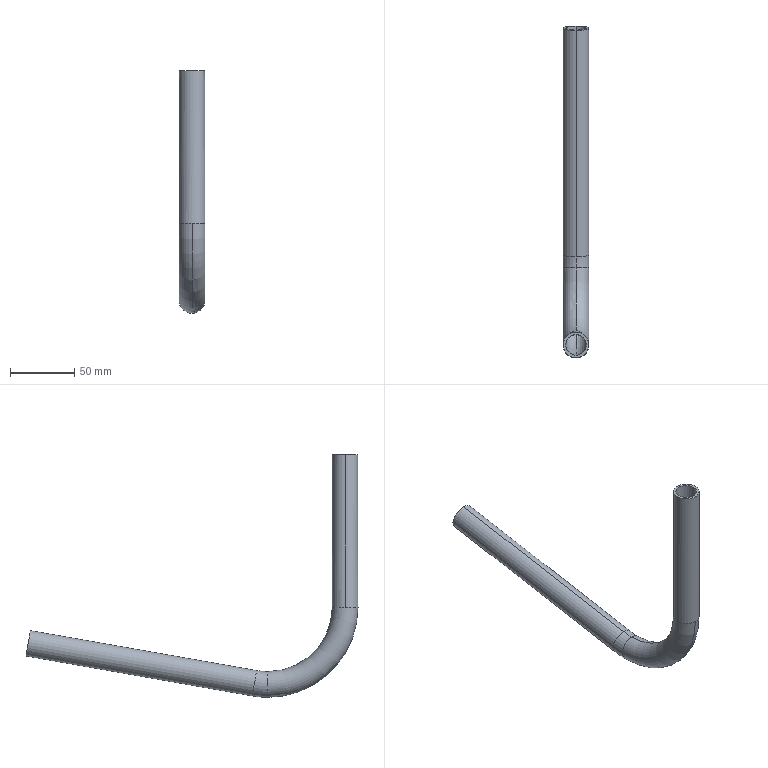Part | STEP file | Handlebar | 1 solid | 18 faces | box 20 x 257.938 x 188.495 mm | volume 45432 mm3 | torus 8 | cylinder 8 | plane 2 | commonest cylinder face diameters 16 x4 20 x4
STEP:
#1=CARTESIAN_POINT('',(0.,0.,0.));
#2=DIRECTION('',(0.,0.,1.));
#3=DIRECTION('',(1.,0.,0.));
#4=AXIS2_PLACEMENT_3D('',#1,#2,#3);
#5=CARTESIAN_POINT('',(0.,8.,-118.495));
#6=VERTEX_POINT('',#5);
#7=CARTESIAN_POINT('',(-8.,0.,-118.495));
#8=VERTEX_POINT('',#7);
#9=CARTESIAN_POINT('',(0.,0.,-118.495));
#10=DIRECTION('',(0.,0.,1.));
#11=DIRECTION('',(1.,0.,0.));
#12=AXIS2_PLACEMENT_3D('',#9,#10,#11);
#13=CIRCLE('',#12,8.);
#14=CARTESIAN_POINT('',(0.,60.,-118.495));
#15=DIRECTION('',(1.,0.,0.));
#16=DIRECTION('',(0.,0.,-1.));
#17=AXIS2_PLACEMENT_3D('',#14,#15,#16);
#18=TOROIDAL_SURFACE('',#17,60.,8.);
#19=CARTESIAN_POINT('',(4.712,1.571));
#20=DIRECTION('',(0.,1.));
#21=VECTOR('',#20,1.);
#22=LINE('',#19,#21);
#23=(GEOMETRIC_REPRESENTATION_CONTEXT(2)PARAMETRIC_REPRESENTATION_CONTEXT()REPRESENTATION_CONTEXT('',''));
#24=DEFINITIONAL_REPRESENTATION('',(#22),#23);
#25=PCURVE('',#18,#24);
#26=CARTESIAN_POINT('',(0.,0.,-118.495));
#27=DIRECTION('',(0.,0.,1.));
#28=DIRECTION('',(1.,0.,0.));
#29=AXIS2_PLACEMENT_3D('',#26,#27,#28);
#30=CYLINDRICAL_SURFACE('',#29,8.);
#31=CARTESIAN_POINT('',(0.,0.));
#32=DIRECTION('',(1.,0.));
#33=VECTOR('',#32,1.);
#34=LINE('',#31,#33);
#35=(GEOMETRIC_REPRESENTATION_CONTEXT(2)PARAMETRIC_REPRESENTATION_CONTEXT()REPRESENTATION_CONTEXT('',''));
#36=DEFINITIONAL_REPRESENTATION('',(#34),#35);
#37=PCURVE('',#30,#36);
#38=SURFACE_CURVE('',#13,(#25,#37),.PCURVE_S1.);
#39=EDGE_CURVE('',#6,#8,#38,.T.);
#40=ORIENTED_EDGE('',*,*,#39,.F.);
#41=CARTESIAN_POINT('',(0.,60.,-170.495));
#42=VERTEX_POINT('',#41);
#43=CARTESIAN_POINT('',(0.,60.,-118.495));
#44=DIRECTION('',(1.,0.,0.));
#45=DIRECTION('',(0.,0.,-1.));
#46=AXIS2_PLACEMENT_3D('',#43,#44,#45);
#47=CIRCLE('',#46,52.);
#48=CARTESIAN_POINT('',(0.,3.142));
#49=DIRECTION('',(1.,0.));
#50=VECTOR('',#49,1.);
#51=LINE('',#48,#50);
#52=(GEOMETRIC_REPRESENTATION_CONTEXT(2)PARAMETRIC_REPRESENTATION_CONTEXT()REPRESENTATION_CONTEXT('',''));
#53=DEFINITIONAL_REPRESENTATION('',(#51),#52);
#54=PCURVE('',#18,#53);
#55=CARTESIAN_POINT('',(0.,60.,-118.495));
#56=DIRECTION('',(1.,0.,0.));
#57=DIRECTION('',(0.,0.,-1.));
#58=AXIS2_PLACEMENT_3D('',#55,#56,#57);
#59=TOROIDAL_SURFACE('',#58,60.,8.);
#60=CARTESIAN_POINT('',(0.,3.142));
#61=DIRECTION('',(1.,0.));
#62=VECTOR('',#61,1.);
#63=LINE('',#60,#62);
#64=(GEOMETRIC_REPRESENTATION_CONTEXT(2)PARAMETRIC_REPRESENTATION_CONTEXT()REPRESENTATION_CONTEXT('',''));
#65=DEFINITIONAL_REPRESENTATION('',(#63),#64);
#66=PCURVE('',#59,#65);
#67=SURFACE_CURVE('',#47,(#54,#66),.PCURVE_S1.);
#68=EDGE_CURVE('',#6,#42,#67,.T.);
#69=ORIENTED_EDGE('',*,*,#68,.T.);
#70=CARTESIAN_POINT('',(0.,60.,-186.495));
#71=VERTEX_POINT('',#70);
#72=CARTESIAN_POINT('',(0.,60.,-178.495));
#73=DIRECTION('',(0.,-1.,0.));
#74=DIRECTION('',(0.,0.,-1.));
#75=AXIS2_PLACEMENT_3D('',#72,#73,#74);
#76=CIRCLE('',#75,8.);
#77=CARTESIAN_POINT('',(6.283,0.));
#78=DIRECTION('',(0.,1.));
#79=VECTOR('',#78,1.);
#80=LINE('',#77,#79);
#81=(GEOMETRIC_REPRESENTATION_CONTEXT(2)PARAMETRIC_REPRESENTATION_CONTEXT()REPRESENTATION_CONTEXT('',''));
#82=DEFINITIONAL_REPRESENTATION('',(#80),#81);
#83=PCURVE('',#18,#82);
#84=CARTESIAN_POINT('',(0.,60.,-118.495));
#85=DIRECTION('',(1.,0.,0.));
#86=DIRECTION('',(0.,0.,-1.));
#87=AXIS2_PLACEMENT_3D('',#84,#85,#86);
#88=TOROIDAL_SURFACE('',#87,60.,8.);
#89=CARTESIAN_POINT('',(0.,0.));
#90=DIRECTION('',(0.,1.));
#91=VECTOR('',#90,1.);
#92=LINE('',#89,#91);
#93=(GEOMETRIC_REPRESENTATION_CONTEXT(2)PARAMETRIC_REPRESENTATION_CONTEXT()REPRESENTATION_CONTEXT('',''));
#94=DEFINITIONAL_REPRESENTATION('',(#92),#93);
#95=PCURVE('',#88,#94);
#96=SURFACE_CURVE('',#76,(#83,#95),.PCURVE_S1.);
#97=EDGE_CURVE('',#42,#71,#96,.T.);
#98=ORIENTED_EDGE('',*,*,#97,.T.);
#99=CARTESIAN_POINT('',(0.,-8.,-118.495));
#100=VERTEX_POINT('',#99);
#101=CARTESIAN_POINT('',(0.,60.,-118.495));
#102=DIRECTION('',(1.,0.,0.));
#103=DIRECTION('',(0.,0.,-1.));
#104=AXIS2_PLACEMENT_3D('',#101,#102,#103);
#105=CIRCLE('',#104,68.);
#106=CARTESIAN_POINT('',(0.,6.283));
#107=DIRECTION('',(1.,0.));
#108=VECTOR('',#107,1.);
#109=LINE('',#106,#108);
#110=(GEOMETRIC_REPRESENTATION_CONTEXT(2)PARAMETRIC_REPRESENTATION_CONTEXT()REPRESENTATION_CONTEXT('',''));
#111=DEFINITIONAL_REPRESENTATION('',(#109),#110);
#112=PCURVE('',#18,#111);
#113=CARTESIAN_POINT('',(0.,0.));
#114=DIRECTION('',(1.,0.));
#115=VECTOR('',#114,1.);
#116=LINE('',#113,#115);
#117=(GEOMETRIC_REPRESENTATION_CONTEXT(2)PARAMETRIC_REPRESENTATION_CONTEXT()REPRESENTATION_CONTEXT('',''));
#118=DEFINITIONAL_REPRESENTATION('',(#116),#117);
#119=PCURVE('',#59,#118);
#120=SURFACE_CURVE('',#105,(#112,#119),.PCURVE_S1.);
#121=EDGE_CURVE('',#100,#71,#120,.T.);
#122=ORIENTED_EDGE('',*,*,#121,.F.);
#123=CARTESIAN_POINT('',(0.,0.,-118.495));
#124=DIRECTION('',(0.,0.,1.));
#125=DIRECTION('',(1.,0.,0.));
#126=AXIS2_PLACEMENT_3D('',#123,#124,#125);
#127=CIRCLE('',#126,8.);
#128=CARTESIAN_POINT('',(4.712,1.571));
#129=DIRECTION('',(0.,1.));
#130=VECTOR('',#129,1.);
#131=LINE('',#128,#130);
#132=(GEOMETRIC_REPRESENTATION_CONTEXT(2)PARAMETRIC_REPRESENTATION_CONTEXT()REPRESENTATION_CONTEXT('',''));
#133=DEFINITIONAL_REPRESENTATION('',(#131),#132);
#134=PCURVE('',#18,#133);
#135=CARTESIAN_POINT('',(0.,0.,-118.495));
#136=DIRECTION('',(0.,0.,1.));
#137=DIRECTION('',(1.,0.,0.));
#138=AXIS2_PLACEMENT_3D('',#135,#136,#137);
#139=CYLINDRICAL_SURFACE('',#138,8.);
#140=CARTESIAN_POINT('',(0.,0.));
#141=DIRECTION('',(1.,0.));
#142=VECTOR('',#141,1.);
#143=LINE('',#140,#142);
#144=(GEOMETRIC_REPRESENTATION_CONTEXT(2)PARAMETRIC_REPRESENTATION_CONTEXT()REPRESENTATION_CONTEXT('',''));
#145=DEFINITIONAL_REPRESENTATION('',(#143),#144);
#146=PCURVE('',#139,#145);
#147=SURFACE_CURVE('',#127,(#134,#146),.PCURVE_S1.);
#148=EDGE_CURVE('',#8,#100,#147,.T.);
#149=ORIENTED_EDGE('',*,*,#148,.F.);
#150=EDGE_LOOP('',(#40,#69,#98,#122,#149));
#151=FACE_BOUND('',#150,.F.);
#152=ADVANCED_FACE('',(#151),#18,.F.);
#153=CARTESIAN_POINT('',(0.,60.,-188.495));
#154=VERTEX_POINT('',#153);
#155=CARTESIAN_POINT('',(0.,60.,-168.495));
#156=VERTEX_POINT('',#155);
#157=CARTESIAN_POINT('',(0.,60.,-178.495));
#158=DIRECTION('',(0.,-1.,0.));
#159=DIRECTION('',(0.,0.,-1.));
#160=AXIS2_PLACEMENT_3D('',#157,#158,#159);
#161=CIRCLE('',#160,10.);
#162=CARTESIAN_POINT('',(0.,60.,-118.495));
#163=DIRECTION('',(1.,0.,0.));
#164=DIRECTION('',(0.,0.,-1.));
#165=AXIS2_PLACEMENT_3D('',#162,#163,#164);
#166=TOROIDAL_SURFACE('',#165,60.,10.);
#167=CARTESIAN_POINT('',(0.,0.));
#168=DIRECTION('',(0.,1.));
#169=VECTOR('',#168,1.);
#170=LINE('',#167,#169);
#171=(GEOMETRIC_REPRESENTATION_CONTEXT(2)PARAMETRIC_REPRESENTATION_CONTEXT()REPRESENTATION_CONTEXT('',''));
#172=DEFINITIONAL_REPRESENTATION('',(#170),#171);
#173=PCURVE('',#166,#172);
#174=CARTESIAN_POINT('',(0.,60.,-118.495));
#175=DIRECTION('',(1.,0.,0.));
#176=DIRECTION('',(0.,0.,-1.));
#177=AXIS2_PLACEMENT_3D('',#174,#175,#176);
#178=TOROIDAL_SURFACE('',#177,60.,10.);
#179=CARTESIAN_POINT('',(6.283,0.));
#180=DIRECTION('',(0.,1.));
#181=VECTOR('',#180,1.);
#182=LINE('',#179,#181);
#183=(GEOMETRIC_REPRESENTATION_CONTEXT(2)PARAMETRIC_REPRESENTATION_CONTEXT()REPRESENTATION_CONTEXT('',''));
#184=DEFINITIONAL_REPRESENTATION('',(#182),#183);
#185=PCURVE('',#178,#184);
#186=SURFACE_CURVE('',#161,(#173,#185),.PCURVE_S1.);
#187=EDGE_CURVE('',#154,#156,#186,.T.);
#188=ORIENTED_EDGE('',*,*,#187,.F.);
#189=CARTESIAN_POINT('',(0.,72.155,-187.431));
#190=VERTEX_POINT('',#189);
#191=CARTESIAN_POINT('',(0.,60.,-118.495));
#192=DIRECTION('',(1.,0.,0.));
#193=DIRECTION('',(0.,0.,-1.));
#194=AXIS2_PLACEMENT_3D('',#191,#192,#193);
#195=CIRCLE('',#194,70.);
#196=CARTESIAN_POINT('',(0.,0.));
#197=DIRECTION('',(1.,0.));
#198=VECTOR('',#197,1.);
#199=LINE('',#196,#198);
#200=(GEOMETRIC_REPRESENTATION_CONTEXT(2)PARAMETRIC_REPRESENTATION_CONTEXT()REPRESENTATION_CONTEXT('',''));
#201=DEFINITIONAL_REPRESENTATION('',(#199),#200);
#202=PCURVE('',#166,#201);
#203=CARTESIAN_POINT('',(0.,60.,-118.495));
#204=DIRECTION('',(1.,0.,0.));
#205=DIRECTION('',(0.,0.,-1.));
#206=AXIS2_PLACEMENT_3D('',#203,#204,#205);
#207=TOROIDAL_SURFACE('',#206,60.,10.);
#208=CARTESIAN_POINT('',(0.,6.283));
#209=DIRECTION('',(1.,0.));
#210=VECTOR('',#209,1.);
#211=LINE('',#208,#210);
#212=(GEOMETRIC_REPRESENTATION_CONTEXT(2)PARAMETRIC_REPRESENTATION_CONTEXT()REPRESENTATION_CONTEXT('',''));
#213=DEFINITIONAL_REPRESENTATION('',(#211),#212);
#214=PCURVE('',#207,#213);
#215=SURFACE_CURVE('',#195,(#202,#214),.PCURVE_S1.);
#216=EDGE_CURVE('',#154,#190,#215,.T.);
#217=ORIENTED_EDGE('',*,*,#216,.T.);
#218=CARTESIAN_POINT('',(0.,68.682,-167.735));
#219=VERTEX_POINT('',#218);
#220=CARTESIAN_POINT('',(0.,70.419,-177.583));
#221=DIRECTION('',(0.,-0.9848,-0.1736));
#222=DIRECTION('',(1.,0.,0.));
#223=AXIS2_PLACEMENT_3D('',#220,#221,#222);
#224=CIRCLE('',#223,10.);
#225=CARTESIAN_POINT('',(0.1745,-4.712));
#226=DIRECTION('',(0.,1.));
#227=VECTOR('',#226,1.);
#228=LINE('',#225,#227);
#229=(GEOMETRIC_REPRESENTATION_CONTEXT(2)PARAMETRIC_REPRESENTATION_CONTEXT()REPRESENTATION_CONTEXT('',''));
#230=DEFINITIONAL_REPRESENTATION('',(#228),#229);
#231=PCURVE('',#166,#230);
#232=CARTESIAN_POINT('',(0.,70.419,-177.583));
#233=DIRECTION('',(0.,0.9848,0.1736));
#234=DIRECTION('',(0.,-0.1736,0.9848));
#235=AXIS2_PLACEMENT_3D('',#232,#233,#234);
#236=CYLINDRICAL_SURFACE('',#235,10.);
#237=CARTESIAN_POINT('',(7.854,0.));
#238=DIRECTION('',(-1.,0.));
#239=VECTOR('',#238,1.);
#240=LINE('',#237,#239);
#241=(GEOMETRIC_REPRESENTATION_CONTEXT(2)PARAMETRIC_REPRESENTATION_CONTEXT()REPRESENTATION_CONTEXT('',''));
#242=DEFINITIONAL_REPRESENTATION('',(#240),#241);
#243=PCURVE('',#236,#242);
#244=SURFACE_CURVE('',#224,(#231,#243),.PCURVE_S1.);
#245=EDGE_CURVE('',#190,#219,#244,.T.);
#246=ORIENTED_EDGE('',*,*,#245,.T.);
#247=CARTESIAN_POINT('',(0.,60.,-118.495));
#248=DIRECTION('',(1.,0.,0.));
#249=DIRECTION('',(0.,0.,-1.));
#250=AXIS2_PLACEMENT_3D('',#247,#248,#249);
#251=CIRCLE('',#250,50.);
#252=CARTESIAN_POINT('',(0.,3.142));
#253=DIRECTION('',(1.,0.));
#254=VECTOR('',#253,1.);
#255=LINE('',#252,#254);
#256=(GEOMETRIC_REPRESENTATION_CONTEXT(2)PARAMETRIC_REPRESENTATION_CONTEXT()REPRESENTATION_CONTEXT('',''));
#257=DEFINITIONAL_REPRESENTATION('',(#255),#256);
#258=PCURVE('',#166,#257);
#259=CARTESIAN_POINT('',(0.,3.142));
#260=DIRECTION('',(1.,0.));
#261=VECTOR('',#260,1.);
#262=LINE('',#259,#261);
#263=(GEOMETRIC_REPRESENTATION_CONTEXT(2)PARAMETRIC_REPRESENTATION_CONTEXT()REPRESENTATION_CONTEXT('',''));
#264=DEFINITIONAL_REPRESENTATION('',(#262),#263);
#265=PCURVE('',#207,#264);
#266=SURFACE_CURVE('',#251,(#258,#265),.PCURVE_S1.);
#267=EDGE_CURVE('',#156,#219,#266,.T.);
#268=ORIENTED_EDGE('',*,*,#267,.F.);
#269=EDGE_LOOP('',(#188,#217,#246,#268));
#270=FACE_BOUND('',#269,.T.);
#271=ADVANCED_FACE('',(#270),#166,.T.);
#272=CARTESIAN_POINT('',(0.,-10.,-118.495));
#273=VERTEX_POINT('',#272);
#274=CARTESIAN_POINT('',(10.,0.,-118.495));
#275=VERTEX_POINT('',#274);
#276=CARTESIAN_POINT('',(0.,0.,-118.495));
#277=DIRECTION('',(0.,0.,1.));
#278=DIRECTION('',(1.,0.,0.));
#279=AXIS2_PLACEMENT_3D('',#276,#277,#278);
#280=CIRCLE('',#279,10.);
#281=CARTESIAN_POINT('',(4.712,-4.712));
#282=DIRECTION('',(0.,1.));
#283=VECTOR('',#282,1.);
#284=LINE('',#281,#283);
#285=(GEOMETRIC_REPRESENTATION_CONTEXT(2)PARAMETRIC_REPRESENTATION_CONTEXT()REPRESENTATION_CONTEXT('',''));
#286=DEFINITIONAL_REPRESENTATION('',(#284),#285);
#287=PCURVE('',#178,#286);
#288=CARTESIAN_POINT('',(0.,0.,-118.495));
#289=DIRECTION('',(0.,0.,1.));
#290=DIRECTION('',(1.,0.,0.));
#291=AXIS2_PLACEMENT_3D('',#288,#289,#290);
#292=CYLINDRICAL_SURFACE('',#291,10.);
#293=CARTESIAN_POINT('',(0.,0.));
#294=DIRECTION('',(1.,0.));
#295=VECTOR('',#294,1.);
#296=LINE('',#293,#295);
#297=(GEOMETRIC_REPRESENTATION_CONTEXT(2)PARAMETRIC_REPRESENTATION_CONTEXT()REPRESENTATION_CONTEXT('',''));
#298=DEFINITIONAL_REPRESENTATION('',(#296),#297);
#299=PCURVE('',#292,#298);
#300=SURFACE_CURVE('',#280,(#287,#299),.PCURVE_S1.);
#301=EDGE_CURVE('',#273,#275,#300,.T.);
#302=ORIENTED_EDGE('',*,*,#301,.F.);
#303=CARTESIAN_POINT('',(0.,60.,-118.495));
#304=DIRECTION('',(1.,0.,0.));
#305=DIRECTION('',(0.,0.,-1.));
#306=AXIS2_PLACEMENT_3D('',#303,#304,#305);
#307=CIRCLE('',#306,70.);
#308=CARTESIAN_POINT('',(0.,0.));
#309=DIRECTION('',(1.,0.));
#310=VECTOR('',#309,1.);
#311=LINE('',#308,#310);
#312=(GEOMETRIC_REPRESENTATION_CONTEXT(2)PARAMETRIC_REPRESENTATION_CONTEXT()REPRESENTATION_CONTEXT('',''));
#313=DEFINITIONAL_REPRESENTATION('',(#311),#312);
#314=PCURVE('',#178,#313);
#315=CARTESIAN_POINT('',(0.,60.,-118.495));
#316=DIRECTION('',(1.,0.,0.));
#317=DIRECTION('',(0.,0.,-1.));
#318=AXIS2_PLACEMENT_3D('',#315,#316,#317);
#319=TOROIDAL_SURFACE('',#318,60.,10.);
#320=CARTESIAN_POINT('',(0.,6.283));
#321=DIRECTION('',(1.,0.));
#322=VECTOR('',#321,1.);
#323=LINE('',#320,#322);
#324=(GEOMETRIC_REPRESENTATION_CONTEXT(2)PARAMETRIC_REPRESENTATION_CONTEXT()REPRESENTATION_CONTEXT('',''));
#325=DEFINITIONAL_REPRESENTATION('',(#323),#324);
#326=PCURVE('',#319,#325);
#327=SURFACE_CURVE('',#307,(#314,#326),.PCURVE_S1.);
#328=EDGE_CURVE('',#273,#154,#327,.T.);
#329=ORIENTED_EDGE('',*,*,#328,.T.);
#330=ORIENTED_EDGE('',*,*,#187,.T.);
#331=CARTESIAN_POINT('',(0.,10.,-118.495));
#332=VERTEX_POINT('',#331);
#333=CARTESIAN_POINT('',(0.,60.,-118.495));
#334=DIRECTION('',(1.,0.,0.));
#335=DIRECTION('',(0.,0.,-1.));
#336=AXIS2_PLACEMENT_3D('',#333,#334,#335);
#337=CIRCLE('',#336,50.);
#338=CARTESIAN_POINT('',(0.,3.142));
#339=DIRECTION('',(1.,0.));
#340=VECTOR('',#339,1.);
#341=LINE('',#338,#340);
#342=(GEOMETRIC_REPRESENTATION_CONTEXT(2)PARAMETRIC_REPRESENTATION_CONTEXT()REPRESENTATION_CONTEXT('',''));
#343=DEFINITIONAL_REPRESENTATION('',(#341),#342);
#344=PCURVE('',#178,#343);
#345=CARTESIAN_POINT('',(0.,3.142));
#346=DIRECTION('',(1.,0.));
#347=VECTOR('',#346,1.);
#348=LINE('',#345,#347);
#349=(GEOMETRIC_REPRESENTATION_CONTEXT(2)PARAMETRIC_REPRESENTATION_CONTEXT()REPRESENTATION_CONTEXT('',''));
#350=DEFINITIONAL_REPRESENTATION('',(#348),#349);
#351=PCURVE('',#319,#350);
#352=SURFACE_CURVE('',#337,(#344,#351),.PCURVE_S1.);
#353=EDGE_CURVE('',#332,#156,#352,.T.);
#354=ORIENTED_EDGE('',*,*,#353,.F.);
#355=CARTESIAN_POINT('',(0.,0.,-118.495));
#356=DIRECTION('',(0.,0.,1.));
#357=DIRECTION('',(1.,0.,0.));
#358=AXIS2_PLACEMENT_3D('',#355,#356,#357);
#359=CIRCLE('',#358,10.);
#360=CARTESIAN_POINT('',(4.712,1.571));
#361=DIRECTION('',(0.,1.));
#362=VECTOR('',#361,1.);
#363=LINE('',#360,#362);
#364=(GEOMETRIC_REPRESENTATION_CONTEXT(2)PARAMETRIC_REPRESENTATION_CONTEXT()REPRESENTATION_CONTEXT('',''));
#365=DEFINITIONAL_REPRESENTATION('',(#363),#364);
#366=PCURVE('',#178,#365);
#367=CARTESIAN_POINT('',(0.,0.,-118.495));
#368=DIRECTION('',(0.,0.,1.));
#369=DIRECTION('',(1.,0.,0.));
#370=AXIS2_PLACEMENT_3D('',#367,#368,#369);
#371=CYLINDRICAL_SURFACE('',#370,10.);
#372=CARTESIAN_POINT('',(0.,0.));
#373=DIRECTION('',(1.,0.));
#374=VECTOR('',#373,1.);
#375=LINE('',#372,#374);
#376=(GEOMETRIC_REPRESENTATION_CONTEXT(2)PARAMETRIC_REPRESENTATION_CONTEXT()REPRESENTATION_CONTEXT('',''));
#377=DEFINITIONAL_REPRESENTATION('',(#375),#376);
#378=PCURVE('',#371,#377);
#379=SURFACE_CURVE('',#359,(#366,#378),.PCURVE_S1.);
#380=EDGE_CURVE('',#275,#332,#379,.T.);
#381=ORIENTED_EDGE('',*,*,#380,.F.);
#382=EDGE_LOOP('',(#302,#329,#330,#354,#381));
#383=FACE_BOUND('',#382,.T.);
#384=ADVANCED_FACE('',(#383),#178,.T.);
#385=CARTESIAN_POINT('',(0.,69.03,-169.705));
#386=VERTEX_POINT('',#385);
#387=CARTESIAN_POINT('',(0.,60.,-118.495));
#388=DIRECTION('',(1.,0.,0.));
#389=DIRECTION('',(0.,0.,-1.));
#390=AXIS2_PLACEMENT_3D('',#387,#388,#389);
#391=CIRCLE('',#390,52.);
#392=CARTESIAN_POINT('',(0.,3.142));
#393=DIRECTION('',(1.,0.));
#394=VECTOR('',#393,1.);
#395=LINE('',#392,#394);
#396=(GEOMETRIC_REPRESENTATION_CONTEXT(2)PARAMETRIC_REPRESENTATION_CONTEXT()REPRESENTATION_CONTEXT('',''));
#397=DEFINITIONAL_REPRESENTATION('',(#395),#396);
#398=PCURVE('',#88,#397);
#399=CARTESIAN_POINT('',(0.,60.,-118.495));
#400=DIRECTION('',(1.,0.,0.));
#401=DIRECTION('',(0.,0.,-1.));
#402=AXIS2_PLACEMENT_3D('',#399,#400,#401);
#403=TOROIDAL_SURFACE('',#402,60.,8.);
#404=CARTESIAN_POINT('',(0.,3.142));
#405=DIRECTION('',(1.,0.));
#406=VECTOR('',#405,1.);
#407=LINE('',#404,#406);
#408=(GEOMETRIC_REPRESENTATION_CONTEXT(2)PARAMETRIC_REPRESENTATION_CONTEXT()REPRESENTATION_CONTEXT('',''));
#409=DEFINITIONAL_REPRESENTATION('',(#407),#408);
#410=PCURVE('',#403,#409);
#411=SURFACE_CURVE('',#391,(#398,#410),.PCURVE_S1.);
#412=EDGE_CURVE('',#42,#386,#411,.T.);
#413=ORIENTED_EDGE('',*,*,#412,.T.);
#414=CARTESIAN_POINT('',(0.,71.808,-185.462));
#415=VERTEX_POINT('',#414);
#416=CARTESIAN_POINT('',(0.,70.419,-177.583));
#417=DIRECTION('',(0.,-0.9848,-0.1736));
#418=DIRECTION('',(1.,0.,0.));
#419=AXIS2_PLACEMENT_3D('',#416,#417,#418);
#420=CIRCLE('',#419,8.);
#421=CARTESIAN_POINT('',(0.1745,1.571));
#422=DIRECTION('',(0.,1.));
#423=VECTOR('',#422,1.);
#424=LINE('',#421,#423);
#425=(GEOMETRIC_REPRESENTATION_CONTEXT(2)PARAMETRIC_REPRESENTATION_CONTEXT()REPRESENTATION_CONTEXT('',''));
#426=DEFINITIONAL_REPRESENTATION('',(#424),#425);
#427=PCURVE('',#88,#426);
#428=CARTESIAN_POINT('',(0.,70.419,-177.583));
#429=DIRECTION('',(0.,0.9848,0.1736));
#430=DIRECTION('',(0.,-0.1736,0.9848));
#431=AXIS2_PLACEMENT_3D('',#428,#429,#430);
#432=CYLINDRICAL_SURFACE('',#431,8.);
#433=CARTESIAN_POINT('',(7.854,0.));
#434=DIRECTION('',(-1.,0.));
#435=VECTOR('',#434,1.);
#436=LINE('',#433,#435);
#437=(GEOMETRIC_REPRESENTATION_CONTEXT(2)PARAMETRIC_REPRESENTATION_CONTEXT()REPRESENTATION_CONTEXT('',''));
#438=DEFINITIONAL_REPRESENTATION('',(#436),#437);
#439=PCURVE('',#432,#438);
#440=SURFACE_CURVE('',#420,(#427,#439),.PCURVE_S1.);
#441=EDGE_CURVE('',#386,#415,#440,.T.);
#442=ORIENTED_EDGE('',*,*,#441,.T.);
#443=CARTESIAN_POINT('',(0.,60.,-118.495));
#444=DIRECTION('',(1.,0.,0.));
#445=DIRECTION('',(0.,0.,-1.));
#446=AXIS2_PLACEMENT_3D('',#443,#444,#445);
#447=CIRCLE('',#446,68.);
#448=CARTESIAN_POINT('',(0.,6.283));
#449=DIRECTION('',(1.,0.));
#450=VECTOR('',#449,1.);
#451=LINE('',#448,#450);
#452=(GEOMETRIC_REPRESENTATION_CONTEXT(2)PARAMETRIC_REPRESENTATION_CONTEXT()REPRESENTATION_CONTEXT('',''));
#453=DEFINITIONAL_REPRESENTATION('',(#451),#452);
#454=PCURVE('',#88,#453);
#455=CARTESIAN_POINT('',(0.,0.));
#456=DIRECTION('',(1.,0.));
#457=VECTOR('',#456,1.);
#458=LINE('',#455,#457);
#459=(GEOMETRIC_REPRESENTATION_CONTEXT(2)PARAMETRIC_REPRESENTATION_CONTEXT()REPRESENTATION_CONTEXT('',''));
#460=DEFINITIONAL_REPRESENTATION('',(#458),#459);
#461=PCURVE('',#403,#460);
#462=SURFACE_CURVE('',#447,(#454,#461),.PCURVE_S1.);
#463=EDGE_CURVE('',#71,#415,#462,.T.);
#464=ORIENTED_EDGE('',*,*,#463,.F.);
#465=ORIENTED_EDGE('',*,*,#97,.F.);
#466=EDGE_LOOP('',(#413,#442,#464,#465));
#467=FACE_BOUND('',#466,.F.);
#468=ADVANCED_FACE('',(#467),#88,.F.);
#469=ORIENTED_EDGE('',*,*,#380,.T.);
#470=CARTESIAN_POINT('',(-10.,0.,-118.495));
#471=VERTEX_POINT('',#470);
#472=CARTESIAN_POINT('',(0.,0.,-118.495));
#473=DIRECTION('',(0.,0.,1.));
#474=DIRECTION('',(1.,0.,0.));
#475=AXIS2_PLACEMENT_3D('',#472,#473,#474);
#476=CIRCLE('',#475,10.);
#477=CARTESIAN_POINT('',(0.,0.));
#478=DIRECTION('',(1.,0.));
#479=VECTOR('',#478,1.);
#480=LINE('',#477,#479);
#481=(GEOMETRIC_REPRESENTATION_CONTEXT(2)PARAMETRIC_REPRESENTATION_CONTEXT()REPRESENTATION_CONTEXT('',''));
#482=DEFINITIONAL_REPRESENTATION('',(#480),#481);
#483=PCURVE('',#371,#482);
#484=CARTESIAN_POINT('',(4.712,1.571));
#485=DIRECTION('',(0.,1.));
#486=VECTOR('',#485,1.);
#487=LINE('',#484,#486);
#488=(GEOMETRIC_REPRESENTATION_CONTEXT(2)PARAMETRIC_REPRESENTATION_CONTEXT()REPRESENTATION_CONTEXT('',''));
#489=DEFINITIONAL_REPRESENTATION('',(#487),#488);
#490=PCURVE('',#319,#489);
#491=SURFACE_CURVE('',#476,(#483,#490),.PCURVE_S1.);
#492=EDGE_CURVE('',#332,#471,#491,.T.);
#493=ORIENTED_EDGE('',*,*,#492,.T.);
#494=CARTESIAN_POINT('',(-10.,0.,0.));
#495=VERTEX_POINT('',#494);
#496=CARTESIAN_POINT('',(-10.,0.,-118.495));
#497=DIRECTION('',(0.,0.,1.));
#498=VECTOR('',#497,1.);
#499=LINE('',#496,#498);
#500=CARTESIAN_POINT('',(3.142,0.));
#501=DIRECTION('',(0.,1.));
#502=VECTOR('',#501,1.);
#503=LINE('',#500,#502);
#504=(GEOMETRIC_REPRESENTATION_CONTEXT(2)PARAMETRIC_REPRESENTATION_CONTEXT()REPRESENTATION_CONTEXT('',''));
#505=DEFINITIONAL_REPRESENTATION('',(#503),#504);
#506=PCURVE('',#371,#505);
#507=CARTESIAN_POINT('',(3.142,0.));
#508=DIRECTION('',(0.,1.));
#509=VECTOR('',#508,1.);
#510=LINE('',#507,#509);
#511=(GEOMETRIC_REPRESENTATION_CONTEXT(2)PARAMETRIC_REPRESENTATION_CONTEXT()REPRESENTATION_CONTEXT('',''));
#512=DEFINITIONAL_REPRESENTATION('',(#510),#511);
#513=PCURVE('',#292,#512);
#514=SURFACE_CURVE('',#499,(#506,#513),.PCURVE_S1.);
#515=EDGE_CURVE('',#471,#495,#514,.T.);
#516=ORIENTED_EDGE('',*,*,#515,.T.);
#517=CARTESIAN_POINT('',(10.,0.,0.));
#518=VERTEX_POINT('',#517);
#519=CARTESIAN_POINT('',(0.,0.,0.));
#520=DIRECTION('',(0.,0.,1.));
#521=DIRECTION('',(1.,0.,0.));
#522=AXIS2_PLACEMENT_3D('',#519,#520,#521);
#523=CIRCLE('',#522,10.);
#524=CARTESIAN_POINT('',(0.,118.495));
#525=DIRECTION('',(1.,0.));
#526=VECTOR('',#525,1.);
#527=LINE('',#524,#526);
#528=(GEOMETRIC_REPRESENTATION_CONTEXT(2)PARAMETRIC_REPRESENTATION_CONTEXT()REPRESENTATION_CONTEXT('',''));
#529=DEFINITIONAL_REPRESENTATION('',(#527),#528);
#530=PCURVE('',#371,#529);
#531=CARTESIAN_POINT('',(0.,0.,0.));
#532=DIRECTION('',(0.,0.,1.));
#533=DIRECTION('',(1.,0.,0.));
#534=AXIS2_PLACEMENT_3D('',#531,#532,#533);
#535=PLANE('',#534);
#536=CARTESIAN_POINT('',(0.,0.));
#537=DIRECTION('',(1.,0.));
#538=AXIS2_PLACEMENT_2D('',#536,#537);
#539=CIRCLE('',#538,10.);
#540=(GEOMETRIC_REPRESENTATION_CONTEXT(2)PARAMETRIC_REPRESENTATION_CONTEXT()REPRESENTATION_CONTEXT('',''));
#541=DEFINITIONAL_REPRESENTATION('',(#539),#540);
#542=PCURVE('',#535,#541);
#543=SURFACE_CURVE('',#523,(#530,#542),.PCURVE_S1.);
#544=EDGE_CURVE('',#518,#495,#543,.T.);
#545=ORIENTED_EDGE('',*,*,#544,.F.);
#546=CARTESIAN_POINT('',(10.,0.,-118.495));
#547=DIRECTION('',(0.,0.,1.));
#548=VECTOR('',#547,1.);
#549=LINE('',#546,#548);
#550=CARTESIAN_POINT('',(0.,0.));
#551=DIRECTION('',(0.,1.));
#552=VECTOR('',#551,1.);
#553=LINE('',#550,#552);
#554=(GEOMETRIC_REPRESENTATION_CONTEXT(2)PARAMETRIC_REPRESENTATION_CONTEXT()REPRESENTATION_CONTEXT('',''));
#555=DEFINITIONAL_REPRESENTATION('',(#553),#554);
#556=PCURVE('',#371,#555);
#557=CARTESIAN_POINT('',(6.283,0.));
#558=DIRECTION('',(0.,1.));
#559=VECTOR('',#558,1.);
#560=LINE('',#557,#559);
#561=(GEOMETRIC_REPRESENTATION_CONTEXT(2)PARAMETRIC_REPRESENTATION_CONTEXT()REPRESENTATION_CONTEXT('',''));
#562=DEFINITIONAL_REPRESENTATION('',(#560),#561);
#563=PCURVE('',#292,#562);
#564=SURFACE_CURVE('',#549,(#556,#563),.PCURVE_S1.);
#565=EDGE_CURVE('',#275,#518,#564,.T.);
#566=ORIENTED_EDGE('',*,*,#565,.F.);
#567=EDGE_LOOP('',(#469,#493,#516,#545,#566));
#568=FACE_BOUND('',#567,.T.);
#569=ADVANCED_FACE('',(#568),#371,.T.);
#570=CARTESIAN_POINT('',(8.,0.,-118.495));
#571=VERTEX_POINT('',#570);
#572=CARTESIAN_POINT('',(0.,0.,-118.495));
#573=DIRECTION('',(0.,0.,1.));
#574=DIRECTION('',(1.,0.,0.));
#575=AXIS2_PLACEMENT_3D('',#572,#573,#574);
#576=CIRCLE('',#575,8.);
#577=CARTESIAN_POINT('',(0.,0.));
#578=DIRECTION('',(1.,0.));
#579=VECTOR('',#578,1.);
#580=LINE('',#577,#579);
#581=(GEOMETRIC_REPRESENTATION_CONTEXT(2)PARAMETRIC_REPRESENTATION_CONTEXT()REPRESENTATION_CONTEXT('',''));
#582=DEFINITIONAL_REPRESENTATION('',(#580),#581);
#583=PCURVE('',#139,#582);
#584=CARTESIAN_POINT('',(4.712,-4.712));
#585=DIRECTION('',(0.,1.));
#586=VECTOR('',#585,1.);
#587=LINE('',#584,#586);
#588=(GEOMETRIC_REPRESENTATION_CONTEXT(2)PARAMETRIC_REPRESENTATION_CONTEXT()REPRESENTATION_CONTEXT('',''));
#589=DEFINITIONAL_REPRESENTATION('',(#587),#588);
#590=PCURVE('',#59,#589);
#591=SURFACE_CURVE('',#576,(#583,#590),.PCURVE_S1.);
#592=EDGE_CURVE('',#100,#571,#591,.T.);
#593=ORIENTED_EDGE('',*,*,#592,.T.);
#594=CARTESIAN_POINT('',(8.,0.,0.));
#595=VERTEX_POINT('',#594);
#596=CARTESIAN_POINT('',(8.,0.,-118.495));
#597=DIRECTION('',(0.,0.,1.));
#598=VECTOR('',#597,1.);
#599=LINE('',#596,#598);
#600=CARTESIAN_POINT('',(6.283,0.));
#601=DIRECTION('',(0.,1.));
#602=VECTOR('',#601,1.);
#603=LINE('',#600,#602);
#604=(GEOMETRIC_REPRESENTATION_CONTEXT(2)PARAMETRIC_REPRESENTATION_CONTEXT()REPRESENTATION_CONTEXT('',''));
#605=DEFINITIONAL_REPRESENTATION('',(#603),#604);
#606=PCURVE('',#139,#605);
#607=CARTESIAN_POINT('',(0.,0.));
#608=DIRECTION('',(0.,1.));
#609=VECTOR('',#608,1.);
#610=LINE('',#607,#609);
#611=(GEOMETRIC_REPRESENTATION_CONTEXT(2)PARAMETRIC_REPRESENTATION_CONTEXT()REPRESENTATION_CONTEXT('',''));
#612=DEFINITIONAL_REPRESENTATION('',(#610),#611);
#613=PCURVE('',#30,#612);
#614=SURFACE_CURVE('',#599,(#606,#613),.PCURVE_S1.);
#615=EDGE_CURVE('',#571,#595,#614,.T.);
#616=ORIENTED_EDGE('',*,*,#615,.T.);
#617=CARTESIAN_POINT('',(-8.,0.,0.));
#618=VERTEX_POINT('',#617);
#619=CARTESIAN_POINT('',(0.,0.,0.));
#620=DIRECTION('',(0.,0.,1.));
#621=DIRECTION('',(1.,0.,0.));
#622=AXIS2_PLACEMENT_3D('',#619,#620,#621);
#623=CIRCLE('',#622,8.);
#624=CARTESIAN_POINT('',(0.,118.495));
#625=DIRECTION('',(1.,0.));
#626=VECTOR('',#625,1.);
#627=LINE('',#624,#626);
#628=(GEOMETRIC_REPRESENTATION_CONTEXT(2)PARAMETRIC_REPRESENTATION_CONTEXT()REPRESENTATION_CONTEXT('',''));
#629=DEFINITIONAL_REPRESENTATION('',(#627),#628);
#630=PCURVE('',#139,#629);
#631=CARTESIAN_POINT('',(0.,0.));
#632=DIRECTION('',(1.,0.));
#633=AXIS2_PLACEMENT_2D('',#631,#632);
#634=CIRCLE('',#633,8.);
#635=(GEOMETRIC_REPRESENTATION_CONTEXT(2)PARAMETRIC_REPRESENTATION_CONTEXT()REPRESENTATION_CONTEXT('',''));
#636=DEFINITIONAL_REPRESENTATION('',(#634),#635);
#637=PCURVE('',#535,#636);
#638=SURFACE_CURVE('',#623,(#630,#637),.PCURVE_S1.);
#639=EDGE_CURVE('',#618,#595,#638,.T.);
#640=ORIENTED_EDGE('',*,*,#639,.F.);
#641=CARTESIAN_POINT('',(-8.,0.,-118.495));
#642=DIRECTION('',(0.,0.,1.));
#643=VECTOR('',#642,1.);
#644=LINE('',#641,#643);
#645=CARTESIAN_POINT('',(3.142,0.));
#646=DIRECTION('',(0.,1.));
#647=VECTOR('',#646,1.);
#648=LINE('',#645,#647);
#649=(GEOMETRIC_REPRESENTATION_CONTEXT(2)PARAMETRIC_REPRESENTATION_CONTEXT()REPRESENTATION_CONTEXT('',''));
#650=DEFINITIONAL_REPRESENTATION('',(#648),#649);
#651=PCURVE('',#139,#650);
#652=CARTESIAN_POINT('',(3.142,0.));
#653=DIRECTION('',(0.,1.));
#654=VECTOR('',#653,1.);
#655=LINE('',#652,#654);
#656=(GEOMETRIC_REPRESENTATION_CONTEXT(2)PARAMETRIC_REPRESENTATION_CONTEXT()REPRESENTATION_CONTEXT('',''));
#657=DEFINITIONAL_REPRESENTATION('',(#655),#656);
#658=PCURVE('',#30,#657);
#659=SURFACE_CURVE('',#644,(#651,#658),.PCURVE_S1.);
#660=EDGE_CURVE('',#8,#618,#659,.T.);
#661=ORIENTED_EDGE('',*,*,#660,.F.);
#662=ORIENTED_EDGE('',*,*,#148,.T.);
#663=EDGE_LOOP('',(#593,#616,#640,#661,#662));
#664=FACE_BOUND('',#663,.F.);
#665=ADVANCED_FACE('',(#664),#139,.F.);
#666=CARTESIAN_POINT('',(0.,70.419,-177.583));
#667=DIRECTION('',(0.,-0.9848,-0.1736));
#668=DIRECTION('',(1.,0.,0.));
#669=AXIS2_PLACEMENT_3D('',#666,#667,#668);
#670=CIRCLE('',#669,8.);
#671=CARTESIAN_POINT('',(0.1745,-4.712));
#672=DIRECTION('',(0.,1.));
#673=VECTOR('',#672,1.);
#674=LINE('',#671,#673);
#675=(GEOMETRIC_REPRESENTATION_CONTEXT(2)PARAMETRIC_REPRESENTATION_CONTEXT()REPRESENTATION_CONTEXT('',''));
#676=DEFINITIONAL_REPRESENTATION('',(#674),#675);
#677=PCURVE('',#403,#676);
#678=CARTESIAN_POINT('',(0.,70.419,-177.583));
#679=DIRECTION('',(0.,0.9848,0.1736));
#680=DIRECTION('',(0.,-0.1736,0.9848));
#681=AXIS2_PLACEMENT_3D('',#678,#679,#680);
#682=CYLINDRICAL_SURFACE('',#681,8.);
#683=CARTESIAN_POINT('',(7.854,0.));
#684=DIRECTION('',(-1.,0.));
#685=VECTOR('',#684,1.);
#686=LINE('',#683,#685);
#687=(GEOMETRIC_REPRESENTATION_CONTEXT(2)PARAMETRIC_REPRESENTATION_CONTEXT()REPRESENTATION_CONTEXT('',''));
#688=DEFINITIONAL_REPRESENTATION('',(#686),#687);
#689=PCURVE('',#682,#688);
#690=SURFACE_CURVE('',#670,(#677,#689),.PCURVE_S1.);
#691=EDGE_CURVE('',#415,#386,#690,.T.);
#692=ORIENTED_EDGE('',*,*,#691,.T.);
#693=ORIENTED_EDGE('',*,*,#412,.F.);
#694=CARTESIAN_POINT('',(0.,60.,-178.495));
#695=DIRECTION('',(0.,-1.,0.));
#696=DIRECTION('',(0.,0.,-1.));
#697=AXIS2_PLACEMENT_3D('',#694,#695,#696);
#698=CIRCLE('',#697,8.);
#699=CARTESIAN_POINT('',(0.,0.));
#700=DIRECTION('',(0.,1.));
#701=VECTOR('',#700,1.);
#702=LINE('',#699,#701);
#703=(GEOMETRIC_REPRESENTATION_CONTEXT(2)PARAMETRIC_REPRESENTATION_CONTEXT()REPRESENTATION_CONTEXT('',''));
#704=DEFINITIONAL_REPRESENTATION('',(#702),#703);
#705=PCURVE('',#403,#704);
#706=CARTESIAN_POINT('',(6.283,0.));
#707=DIRECTION('',(0.,1.));
#708=VECTOR('',#707,1.);
#709=LINE('',#706,#708);
#710=(GEOMETRIC_REPRESENTATION_CONTEXT(2)PARAMETRIC_REPRESENTATION_CONTEXT()REPRESENTATION_CONTEXT('',''));
#711=DEFINITIONAL_REPRESENTATION('',(#709),#710);
#712=PCURVE('',#59,#711);
#713=SURFACE_CURVE('',#698,(#705,#712),.PCURVE_S1.);
#714=EDGE_CURVE('',#71,#42,#713,.T.);
#715=ORIENTED_EDGE('',*,*,#714,.F.);
#716=ORIENTED_EDGE('',*,*,#463,.T.);
#717=EDGE_LOOP('',(#692,#693,#715,#716));
#718=FACE_BOUND('',#717,.F.);
#719=ADVANCED_FACE('',(#718),#403,.F.);
#720=ORIENTED_EDGE('',*,*,#328,.F.);
#721=CARTESIAN_POINT('',(0.,0.,-118.495));
#722=DIRECTION('',(0.,0.,1.));
#723=DIRECTION('',(1.,0.,0.));
#724=AXIS2_PLACEMENT_3D('',#721,#722,#723);
#725=CIRCLE('',#724,10.);
#726=CARTESIAN_POINT('',(4.712,1.571));
#727=DIRECTION('',(0.,1.));
#728=VECTOR('',#727,1.);
#729=LINE('',#726,#728);
#730=(GEOMETRIC_REPRESENTATION_CONTEXT(2)PARAMETRIC_REPRESENTATION_CONTEXT()REPRESENTATION_CONTEXT('',''));
#731=DEFINITIONAL_REPRESENTATION('',(#729),#730);
#732=PCURVE('',#319,#731);
#733=CARTESIAN_POINT('',(0.,0.));
#734=DIRECTION('',(1.,0.));
#735=VECTOR('',#734,1.);
#736=LINE('',#733,#735);
#737=(GEOMETRIC_REPRESENTATION_CONTEXT(2)PARAMETRIC_REPRESENTATION_CONTEXT()REPRESENTATION_CONTEXT('',''));
#738=DEFINITIONAL_REPRESENTATION('',(#736),#737);
#739=PCURVE('',#292,#738);
#740=SURFACE_CURVE('',#725,(#732,#739),.PCURVE_S1.);
#741=EDGE_CURVE('',#471,#273,#740,.T.);
#742=ORIENTED_EDGE('',*,*,#741,.F.);
#743=ORIENTED_EDGE('',*,*,#492,.F.);
#744=ORIENTED_EDGE('',*,*,#353,.T.);
#745=CARTESIAN_POINT('',(0.,60.,-178.495));
#746=DIRECTION('',(0.,-1.,0.));
#747=DIRECTION('',(0.,0.,-1.));
#748=AXIS2_PLACEMENT_3D('',#745,#746,#747);
#749=CIRCLE('',#748,10.);
#750=CARTESIAN_POINT('',(6.283,0.));
#751=DIRECTION('',(0.,1.));
#752=VECTOR('',#751,1.);
#753=LINE('',#750,#752);
#754=(GEOMETRIC_REPRESENTATION_CONTEXT(2)PARAMETRIC_REPRESENTATION_CONTEXT()REPRESENTATION_CONTEXT('',''));
#755=DEFINITIONAL_REPRESENTATION('',(#753),#754);
#756=PCURVE('',#319,#755);
#757=CARTESIAN_POINT('',(0.,0.));
#758=DIRECTION('',(0.,1.));
#759=VECTOR('',#758,1.);
#760=LINE('',#757,#759);
#761=(GEOMETRIC_REPRESENTATION_CONTEXT(2)PARAMETRIC_REPRESENTATION_CONTEXT()REPRESENTATION_CONTEXT('',''));
#762=DEFINITIONAL_REPRESENTATION('',(#760),#761);
#763=PCURVE('',#207,#762);
#764=SURFACE_CURVE('',#749,(#756,#763),.PCURVE_S1.);
#765=EDGE_CURVE('',#156,#154,#764,.T.);
#766=ORIENTED_EDGE('',*,*,#765,.T.);
#767=EDGE_LOOP('',(#720,#742,#743,#744,#766));
#768=FACE_BOUND('',#767,.T.);
#769=ADVANCED_FACE('',(#768),#319,.T.);
#770=CARTESIAN_POINT('',(0.,244.813,-138.709));
#771=VERTEX_POINT('',#770);
#772=CARTESIAN_POINT('',(0.,69.03,-169.705));
#773=DIRECTION('',(0.,0.9848,0.1736));
#774=VECTOR('',#773,1.);
#775=LINE('',#772,#774);
#776=CARTESIAN_POINT('',(6.283,0.));
#777=DIRECTION('',(0.,1.));
#778=VECTOR('',#777,1.);
#779=LINE('',#776,#778);
#780=(GEOMETRIC_REPRESENTATION_CONTEXT(2)PARAMETRIC_REPRESENTATION_CONTEXT()REPRESENTATION_CONTEXT('',''));
#781=DEFINITIONAL_REPRESENTATION('',(#779),#780);
#782=PCURVE('',#432,#781);
#783=CARTESIAN_POINT('',(0.,0.));
#784=DIRECTION('',(0.,1.));
#785=VECTOR('',#784,1.);
#786=LINE('',#783,#785);
#787=(GEOMETRIC_REPRESENTATION_CONTEXT(2)PARAMETRIC_REPRESENTATION_CONTEXT()REPRESENTATION_CONTEXT('',''));
#788=DEFINITIONAL_REPRESENTATION('',(#786),#787);
#789=PCURVE('',#682,#788);
#790=SURFACE_CURVE('',#775,(#782,#789),.PCURVE_S1.);
#791=EDGE_CURVE('',#386,#771,#790,.T.);
#792=ORIENTED_EDGE('',*,*,#791,.T.);
#793=CARTESIAN_POINT('',(0.,247.591,-154.466));
#794=VERTEX_POINT('',#793);
#795=CARTESIAN_POINT('',(0.,246.202,-146.588));
#796=DIRECTION('',(0.,-0.9848,-0.1736));
#797=DIRECTION('',(1.,0.,0.));
#798=AXIS2_PLACEMENT_3D('',#795,#796,#797);
#799=CIRCLE('',#798,8.);
#800=CARTESIAN_POINT('',(7.854,178.495));
#801=DIRECTION('',(-1.,0.));
#802=VECTOR('',#801,1.);
#803=LINE('',#800,#802);
#804=(GEOMETRIC_REPRESENTATION_CONTEXT(2)PARAMETRIC_REPRESENTATION_CONTEXT()REPRESENTATION_CONTEXT('',''));
#805=DEFINITIONAL_REPRESENTATION('',(#803),#804);
#806=PCURVE('',#432,#805);
#807=CARTESIAN_POINT('',(0.,246.202,-146.588));
#808=DIRECTION('',(0.,-0.9848,-0.1736));
#809=DIRECTION('',(1.,0.,0.));
#810=AXIS2_PLACEMENT_3D('',#807,#808,#809);
#811=PLANE('',#810);
#812=CARTESIAN_POINT('',(0.,0.));
#813=DIRECTION('',(1.,0.));
#814=AXIS2_PLACEMENT_2D('',#812,#813);
#815=CIRCLE('',#814,8.);
#816=(GEOMETRIC_REPRESENTATION_CONTEXT(2)PARAMETRIC_REPRESENTATION_CONTEXT()REPRESENTATION_CONTEXT('',''));
#817=DEFINITIONAL_REPRESENTATION('',(#815),#816);
#818=PCURVE('',#811,#817);
#819=SURFACE_CURVE('',#799,(#806,#818),.PCURVE_S1.);
#820=EDGE_CURVE('',#771,#794,#819,.T.);
#821=ORIENTED_EDGE('',*,*,#820,.T.);
#822=CARTESIAN_POINT('',(0.,71.808,-185.462));
#823=DIRECTION('',(0.,0.9848,0.1736));
#824=VECTOR('',#823,1.);
#825=LINE('',#822,#824);
#826=CARTESIAN_POINT('',(3.142,0.));
#827=DIRECTION('',(0.,1.));
#828=VECTOR('',#827,1.);
#829=LINE('',#826,#828);
#830=(GEOMETRIC_REPRESENTATION_CONTEXT(2)PARAMETRIC_REPRESENTATION_CONTEXT()REPRESENTATION_CONTEXT('',''));
#831=DEFINITIONAL_REPRESENTATION('',(#829),#830);
#832=PCURVE('',#432,#831);
#833=CARTESIAN_POINT('',(3.142,0.));
#834=DIRECTION('',(0.,1.));
#835=VECTOR('',#834,1.);
#836=LINE('',#833,#835);
#837=(GEOMETRIC_REPRESENTATION_CONTEXT(2)PARAMETRIC_REPRESENTATION_CONTEXT()REPRESENTATION_CONTEXT('',''));
#838=DEFINITIONAL_REPRESENTATION('',(#836),#837);
#839=PCURVE('',#682,#838);
#840=SURFACE_CURVE('',#825,(#832,#839),.PCURVE_S1.);
#841=EDGE_CURVE('',#415,#794,#840,.T.);
#842=ORIENTED_EDGE('',*,*,#841,.F.);
#843=ORIENTED_EDGE('',*,*,#441,.F.);
#844=EDGE_LOOP('',(#792,#821,#842,#843));
#845=FACE_BOUND('',#844,.F.);
#846=ADVANCED_FACE('',(#845),#432,.F.);
#847=ORIENTED_EDGE('',*,*,#245,.F.);
#848=CARTESIAN_POINT('',(0.,247.938,-156.436));
#849=VERTEX_POINT('',#848);
#850=CARTESIAN_POINT('',(0.,72.155,-187.431));
#851=DIRECTION('',(0.,0.9848,0.1736));
#852=VECTOR('',#851,1.);
#853=LINE('',#850,#852);
#854=CARTESIAN_POINT('',(3.142,0.));
#855=DIRECTION('',(0.,1.));
#856=VECTOR('',#855,1.);
#857=LINE('',#854,#856);
#858=(GEOMETRIC_REPRESENTATION_CONTEXT(2)PARAMETRIC_REPRESENTATION_CONTEXT()REPRESENTATION_CONTEXT('',''));
#859=DEFINITIONAL_REPRESENTATION('',(#857),#858);
#860=PCURVE('',#236,#859);
#861=CARTESIAN_POINT('',(0.,70.419,-177.583));
#862=DIRECTION('',(0.,0.9848,0.1736));
#863=DIRECTION('',(0.,-0.1736,0.9848));
#864=AXIS2_PLACEMENT_3D('',#861,#862,#863);
#865=CYLINDRICAL_SURFACE('',#864,10.);
#866=CARTESIAN_POINT('',(3.142,0.));
#867=DIRECTION('',(0.,1.));
#868=VECTOR('',#867,1.);
#869=LINE('',#866,#868);
#870=(GEOMETRIC_REPRESENTATION_CONTEXT(2)PARAMETRIC_REPRESENTATION_CONTEXT()REPRESENTATION_CONTEXT('',''));
#871=DEFINITIONAL_REPRESENTATION('',(#869),#870);
#872=PCURVE('',#865,#871);
#873=SURFACE_CURVE('',#853,(#860,#872),.PCURVE_S1.);
#874=EDGE_CURVE('',#190,#849,#873,.T.);
#875=ORIENTED_EDGE('',*,*,#874,.T.);
#876=CARTESIAN_POINT('',(0.,244.465,-136.74));
#877=VERTEX_POINT('',#876);
#878=CARTESIAN_POINT('',(0.,246.202,-146.588));
#879=DIRECTION('',(0.,-0.9848,-0.1736));
#880=DIRECTION('',(1.,0.,0.));
#881=AXIS2_PLACEMENT_3D('',#878,#879,#880);
#882=CIRCLE('',#881,10.);
#883=CARTESIAN_POINT('',(7.854,178.495));
#884=DIRECTION('',(-1.,0.));
#885=VECTOR('',#884,1.);
#886=LINE('',#883,#885);
#887=(GEOMETRIC_REPRESENTATION_CONTEXT(2)PARAMETRIC_REPRESENTATION_CONTEXT()REPRESENTATION_CONTEXT('',''));
#888=DEFINITIONAL_REPRESENTATION('',(#886),#887);
#889=PCURVE('',#236,#888);
#890=CARTESIAN_POINT('',(0.,0.));
#891=DIRECTION('',(1.,0.));
#892=AXIS2_PLACEMENT_2D('',#890,#891);
#893=CIRCLE('',#892,10.);
#894=(GEOMETRIC_REPRESENTATION_CONTEXT(2)PARAMETRIC_REPRESENTATION_CONTEXT()REPRESENTATION_CONTEXT('',''));
#895=DEFINITIONAL_REPRESENTATION('',(#893),#894);
#896=PCURVE('',#811,#895);
#897=SURFACE_CURVE('',#882,(#889,#896),.PCURVE_S1.);
#898=EDGE_CURVE('',#849,#877,#897,.T.);
#899=ORIENTED_EDGE('',*,*,#898,.T.);
#900=CARTESIAN_POINT('',(0.,68.682,-167.735));
#901=DIRECTION('',(0.,0.9848,0.1736));
#902=VECTOR('',#901,1.);
#903=LINE('',#900,#902);
#904=CARTESIAN_POINT('',(0.,0.));
#905=DIRECTION('',(0.,1.));
#906=VECTOR('',#905,1.);
#907=LINE('',#904,#906);
#908=(GEOMETRIC_REPRESENTATION_CONTEXT(2)PARAMETRIC_REPRESENTATION_CONTEXT()REPRESENTATION_CONTEXT('',''));
#909=DEFINITIONAL_REPRESENTATION('',(#907),#908);
#910=PCURVE('',#236,#909);
#911=CARTESIAN_POINT('',(6.283,0.));
#912=DIRECTION('',(0.,1.));
#913=VECTOR('',#912,1.);
#914=LINE('',#911,#913);
#915=(GEOMETRIC_REPRESENTATION_CONTEXT(2)PARAMETRIC_REPRESENTATION_CONTEXT()REPRESENTATION_CONTEXT('',''));
#916=DEFINITIONAL_REPRESENTATION('',(#914),#915);
#917=PCURVE('',#865,#916);
#918=SURFACE_CURVE('',#903,(#910,#917),.PCURVE_S1.);
#919=EDGE_CURVE('',#219,#877,#918,.T.);
#920=ORIENTED_EDGE('',*,*,#919,.F.);
#921=EDGE_LOOP('',(#847,#875,#899,#920));
#922=FACE_BOUND('',#921,.T.);
#923=ADVANCED_FACE('',(#922),#236,.T.);
#924=ORIENTED_EDGE('',*,*,#874,.F.);
#925=CARTESIAN_POINT('',(0.,70.419,-177.583));
#926=DIRECTION('',(0.,-0.9848,-0.1736));
#927=DIRECTION('',(1.,0.,0.));
#928=AXIS2_PLACEMENT_3D('',#925,#926,#927);
#929=CIRCLE('',#928,10.);
#930=CARTESIAN_POINT('',(7.854,0.));
#931=DIRECTION('',(-1.,0.));
#932=VECTOR('',#931,1.);
#933=LINE('',#930,#932);
#934=(GEOMETRIC_REPRESENTATION_CONTEXT(2)PARAMETRIC_REPRESENTATION_CONTEXT()REPRESENTATION_CONTEXT('',''));
#935=DEFINITIONAL_REPRESENTATION('',(#933),#934);
#936=PCURVE('',#865,#935);
#937=CARTESIAN_POINT('',(0.1745,1.571));
#938=DIRECTION('',(0.,1.));
#939=VECTOR('',#938,1.);
#940=LINE('',#937,#939);
#941=(GEOMETRIC_REPRESENTATION_CONTEXT(2)PARAMETRIC_REPRESENTATION_CONTEXT()REPRESENTATION_CONTEXT('',''));
#942=DEFINITIONAL_REPRESENTATION('',(#940),#941);
#943=PCURVE('',#207,#942);
#944=SURFACE_CURVE('',#929,(#936,#943),.PCURVE_S1.);
#945=EDGE_CURVE('',#219,#190,#944,.T.);
#946=ORIENTED_EDGE('',*,*,#945,.F.);
#947=ORIENTED_EDGE('',*,*,#919,.T.);
#948=CARTESIAN_POINT('',(0.,246.202,-146.588));
#949=DIRECTION('',(0.,-0.9848,-0.1736));
#950=DIRECTION('',(1.,0.,0.));
#951=AXIS2_PLACEMENT_3D('',#948,#949,#950);
#952=CIRCLE('',#951,10.);
#953=CARTESIAN_POINT('',(7.854,178.495));
#954=DIRECTION('',(-1.,0.));
#955=VECTOR('',#954,1.);
#956=LINE('',#953,#955);
#957=(GEOMETRIC_REPRESENTATION_CONTEXT(2)PARAMETRIC_REPRESENTATION_CONTEXT()REPRESENTATION_CONTEXT('',''));
#958=DEFINITIONAL_REPRESENTATION('',(#956),#957);
#959=PCURVE('',#865,#958);
#960=CARTESIAN_POINT('',(0.,0.));
#961=DIRECTION('',(1.,0.));
#962=AXIS2_PLACEMENT_2D('',#960,#961);
#963=CIRCLE('',#962,10.);
#964=(GEOMETRIC_REPRESENTATION_CONTEXT(2)PARAMETRIC_REPRESENTATION_CONTEXT()REPRESENTATION_CONTEXT('',''));
#965=DEFINITIONAL_REPRESENTATION('',(#963),#964);
#966=PCURVE('',#811,#965);
#967=SURFACE_CURVE('',#952,(#959,#966),.PCURVE_S1.);
#968=EDGE_CURVE('',#877,#849,#967,.T.);
#969=ORIENTED_EDGE('',*,*,#968,.T.);
#970=EDGE_LOOP('',(#924,#946,#947,#969));
#971=FACE_BOUND('',#970,.T.);
#972=ADVANCED_FACE('',(#971),#865,.T.);
#973=CARTESIAN_POINT('',(0.,246.202,-146.588));
#974=DIRECTION('',(0.,-0.9848,-0.1736));
#975=DIRECTION('',(1.,0.,0.));
#976=AXIS2_PLACEMENT_3D('',#973,#974,#975);
#977=CIRCLE('',#976,8.);
#978=CARTESIAN_POINT('',(7.854,178.495));
#979=DIRECTION('',(-1.,0.));
#980=VECTOR('',#979,1.);
#981=LINE('',#978,#980);
#982=(GEOMETRIC_REPRESENTATION_CONTEXT(2)PARAMETRIC_REPRESENTATION_CONTEXT()REPRESENTATION_CONTEXT('',''));
#983=DEFINITIONAL_REPRESENTATION('',(#981),#982);
#984=PCURVE('',#682,#983);
#985=CARTESIAN_POINT('',(0.,0.));
#986=DIRECTION('',(1.,0.));
#987=AXIS2_PLACEMENT_2D('',#985,#986);
#988=CIRCLE('',#987,8.);
#989=(GEOMETRIC_REPRESENTATION_CONTEXT(2)PARAMETRIC_REPRESENTATION_CONTEXT()REPRESENTATION_CONTEXT('',''));
#990=DEFINITIONAL_REPRESENTATION('',(#988),#989);
#991=PCURVE('',#811,#990);
#992=SURFACE_CURVE('',#977,(#984,#991),.PCURVE_S1.);
#993=EDGE_CURVE('',#794,#771,#992,.T.);
#994=ORIENTED_EDGE('',*,*,#993,.T.);
#995=ORIENTED_EDGE('',*,*,#791,.F.);
#996=ORIENTED_EDGE('',*,*,#691,.F.);
#997=ORIENTED_EDGE('',*,*,#841,.T.);
#998=EDGE_LOOP('',(#994,#995,#996,#997));
#999=FACE_BOUND('',#998,.F.);
#1000=ADVANCED_FACE('',(#999),#682,.F.);
#1001=ORIENTED_EDGE('',*,*,#216,.F.);
#1002=ORIENTED_EDGE('',*,*,#765,.F.);
#1003=ORIENTED_EDGE('',*,*,#267,.T.);
#1004=ORIENTED_EDGE('',*,*,#945,.T.);
#1005=EDGE_LOOP('',(#1001,#1002,#1003,#1004));
#1006=FACE_BOUND('',#1005,.T.);
#1007=ADVANCED_FACE('',(#1006),#207,.T.);
#1008=ORIENTED_EDGE('',*,*,#714,.T.);
#1009=ORIENTED_EDGE('',*,*,#68,.F.);
#1010=CARTESIAN_POINT('',(0.,0.,-118.495));
#1011=DIRECTION('',(0.,0.,1.));
#1012=DIRECTION('',(1.,0.,0.));
#1013=AXIS2_PLACEMENT_3D('',#1010,#1011,#1012);
#1014=CIRCLE('',#1013,8.);
#1015=CARTESIAN_POINT('',(4.712,1.571));
#1016=DIRECTION('',(0.,1.));
#1017=VECTOR('',#1016,1.);
#1018=LINE('',#1015,#1017);
#1019=(GEOMETRIC_REPRESENTATION_CONTEXT(2)PARAMETRIC_REPRESENTATION_CONTEXT()REPRESENTATION_CONTEXT('',''));
#1020=DEFINITIONAL_REPRESENTATION('',(#1018),#1019);
#1021=PCURVE('',#59,#1020);
#1022=CARTESIAN_POINT('',(0.,0.));
#1023=DIRECTION('',(1.,0.));
#1024=VECTOR('',#1023,1.);
#1025=LINE('',#1022,#1024);
#1026=(GEOMETRIC_REPRESENTATION_CONTEXT(2)PARAMETRIC_REPRESENTATION_CONTEXT()REPRESENTATION_CONTEXT('',''));
#1027=DEFINITIONAL_REPRESENTATION('',(#1025),#1026);
#1028=PCURVE('',#30,#1027);
#1029=SURFACE_CURVE('',#1014,(#1021,#1028),.PCURVE_S1.);
#1030=EDGE_CURVE('',#571,#6,#1029,.T.);
#1031=ORIENTED_EDGE('',*,*,#1030,.F.);
#1032=ORIENTED_EDGE('',*,*,#592,.F.);
#1033=ORIENTED_EDGE('',*,*,#121,.T.);
#1034=EDGE_LOOP('',(#1008,#1009,#1031,#1032,#1033));
#1035=FACE_BOUND('',#1034,.F.);
#1036=ADVANCED_FACE('',(#1035),#59,.F.);
#1037=CARTESIAN_POINT('',(0.,0.,0.));
#1038=DIRECTION('',(0.,0.,1.));
#1039=DIRECTION('',(1.,0.,0.));
#1040=AXIS2_PLACEMENT_3D('',#1037,#1038,#1039);
#1041=CIRCLE('',#1040,8.);
#1042=CARTESIAN_POINT('',(0.,118.495));
#1043=DIRECTION('',(1.,0.));
#1044=VECTOR('',#1043,1.);
#1045=LINE('',#1042,#1044);
#1046=(GEOMETRIC_REPRESENTATION_CONTEXT(2)PARAMETRIC_REPRESENTATION_CONTEXT()REPRESENTATION_CONTEXT('',''));
#1047=DEFINITIONAL_REPRESENTATION('',(#1045),#1046);
#1048=PCURVE('',#30,#1047);
#1049=CARTESIAN_POINT('',(0.,0.));
#1050=DIRECTION('',(1.,0.));
#1051=AXIS2_PLACEMENT_2D('',#1049,#1050);
#1052=CIRCLE('',#1051,8.);
#1053=(GEOMETRIC_REPRESENTATION_CONTEXT(2)PARAMETRIC_REPRESENTATION_CONTEXT()REPRESENTATION_CONTEXT('',''));
#1054=DEFINITIONAL_REPRESENTATION('',(#1052),#1053);
#1055=PCURVE('',#535,#1054);
#1056=SURFACE_CURVE('',#1041,(#1048,#1055),.PCURVE_S1.);
#1057=EDGE_CURVE('',#595,#618,#1056,.T.);
#1058=ORIENTED_EDGE('',*,*,#1057,.F.);
#1059=ORIENTED_EDGE('',*,*,#615,.F.);
#1060=ORIENTED_EDGE('',*,*,#1030,.T.);
#1061=ORIENTED_EDGE('',*,*,#39,.T.);
#1062=ORIENTED_EDGE('',*,*,#660,.T.);
#1063=EDGE_LOOP('',(#1058,#1059,#1060,#1061,#1062));
#1064=FACE_BOUND('',#1063,.F.);
#1065=ADVANCED_FACE('',(#1064),#30,.F.);
#1066=ORIENTED_EDGE('',*,*,#515,.F.);
#1067=ORIENTED_EDGE('',*,*,#741,.T.);
#1068=ORIENTED_EDGE('',*,*,#301,.T.);
#1069=ORIENTED_EDGE('',*,*,#565,.T.);
#1070=CARTESIAN_POINT('',(0.,0.,0.));
#1071=DIRECTION('',(0.,0.,1.));
#1072=DIRECTION('',(1.,0.,0.));
#1073=AXIS2_PLACEMENT_3D('',#1070,#1071,#1072);
#1074=CIRCLE('',#1073,10.);
#1075=CARTESIAN_POINT('',(0.,118.495));
#1076=DIRECTION('',(1.,0.));
#1077=VECTOR('',#1076,1.);
#1078=LINE('',#1075,#1077);
#1079=(GEOMETRIC_REPRESENTATION_CONTEXT(2)PARAMETRIC_REPRESENTATION_CONTEXT()REPRESENTATION_CONTEXT('',''));
#1080=DEFINITIONAL_REPRESENTATION('',(#1078),#1079);
#1081=PCURVE('',#292,#1080);
#1082=CARTESIAN_POINT('',(0.,0.));
#1083=DIRECTION('',(1.,0.));
#1084=AXIS2_PLACEMENT_2D('',#1082,#1083);
#1085=CIRCLE('',#1084,10.);
#1086=(GEOMETRIC_REPRESENTATION_CONTEXT(2)PARAMETRIC_REPRESENTATION_CONTEXT()REPRESENTATION_CONTEXT('',''));
#1087=DEFINITIONAL_REPRESENTATION('',(#1085),#1086);
#1088=PCURVE('',#535,#1087);
#1089=SURFACE_CURVE('',#1074,(#1081,#1088),.PCURVE_S1.);
#1090=EDGE_CURVE('',#495,#518,#1089,.T.);
#1091=ORIENTED_EDGE('',*,*,#1090,.F.);
#1092=EDGE_LOOP('',(#1066,#1067,#1068,#1069,#1091));
#1093=FACE_BOUND('',#1092,.T.);
#1094=ADVANCED_FACE('',(#1093),#292,.T.);
#1095=ORIENTED_EDGE('',*,*,#820,.T.);
#1096=ORIENTED_EDGE('',*,*,#993,.T.);
#1097=EDGE_LOOP('',(#1095,#1096));
#1098=FACE_BOUND('',#1097,.T.);
#1099=ORIENTED_EDGE('',*,*,#968,.F.);
#1100=ORIENTED_EDGE('',*,*,#898,.F.);
#1101=EDGE_LOOP('',(#1099,#1100));
#1102=FACE_BOUND('',#1101,.T.);
#1103=ADVANCED_FACE('',(#1098,#1102),#811,.F.);
#1104=ORIENTED_EDGE('',*,*,#1057,.F.);
#1105=ORIENTED_EDGE('',*,*,#639,.F.);
#1106=EDGE_LOOP('',(#1104,#1105));
#1107=FACE_BOUND('',#1106,.T.);
#1108=ORIENTED_EDGE('',*,*,#544,.T.);
#1109=ORIENTED_EDGE('',*,*,#1090,.T.);
#1110=EDGE_LOOP('',(#1108,#1109));
#1111=FACE_BOUND('',#1110,.T.);
#1112=ADVANCED_FACE('',(#1107,#1111),#535,.T.);
#1113=CLOSED_SHELL('',(#152,#271,#384,#468,#569,#665,#719,#769,#846,#923,#972,#1000,#1007,#1036,#1065,#1094,#1103,#1112));
#1114=MANIFOLD_SOLID_BREP('',#1113);
#1115=(LENGTH_UNIT()NAMED_UNIT(*)SI_UNIT(.MILLI.,.METRE.));
#1116=UNCERTAINTY_MEASURE_WITH_UNIT(LENGTH_MEASURE(0.0000001),#1115,'','');
#1117=(NAMED_UNIT(*)PLANE_ANGLE_UNIT()SI_UNIT($,.RADIAN.));
#1118=(NAMED_UNIT(*)SI_UNIT($,.STERADIAN.)SOLID_ANGLE_UNIT());
#1119=(GEOMETRIC_REPRESENTATION_CONTEXT(3)GLOBAL_UNCERTAINTY_ASSIGNED_CONTEXT((#1116))GLOBAL_UNIT_ASSIGNED_CONTEXT((#1115,#1117,#1118))REPRESENTATION_CONTEXT('',''));
#1120=ADVANCED_BREP_SHAPE_REPRESENTATION('',(#4,#1114),#1119);